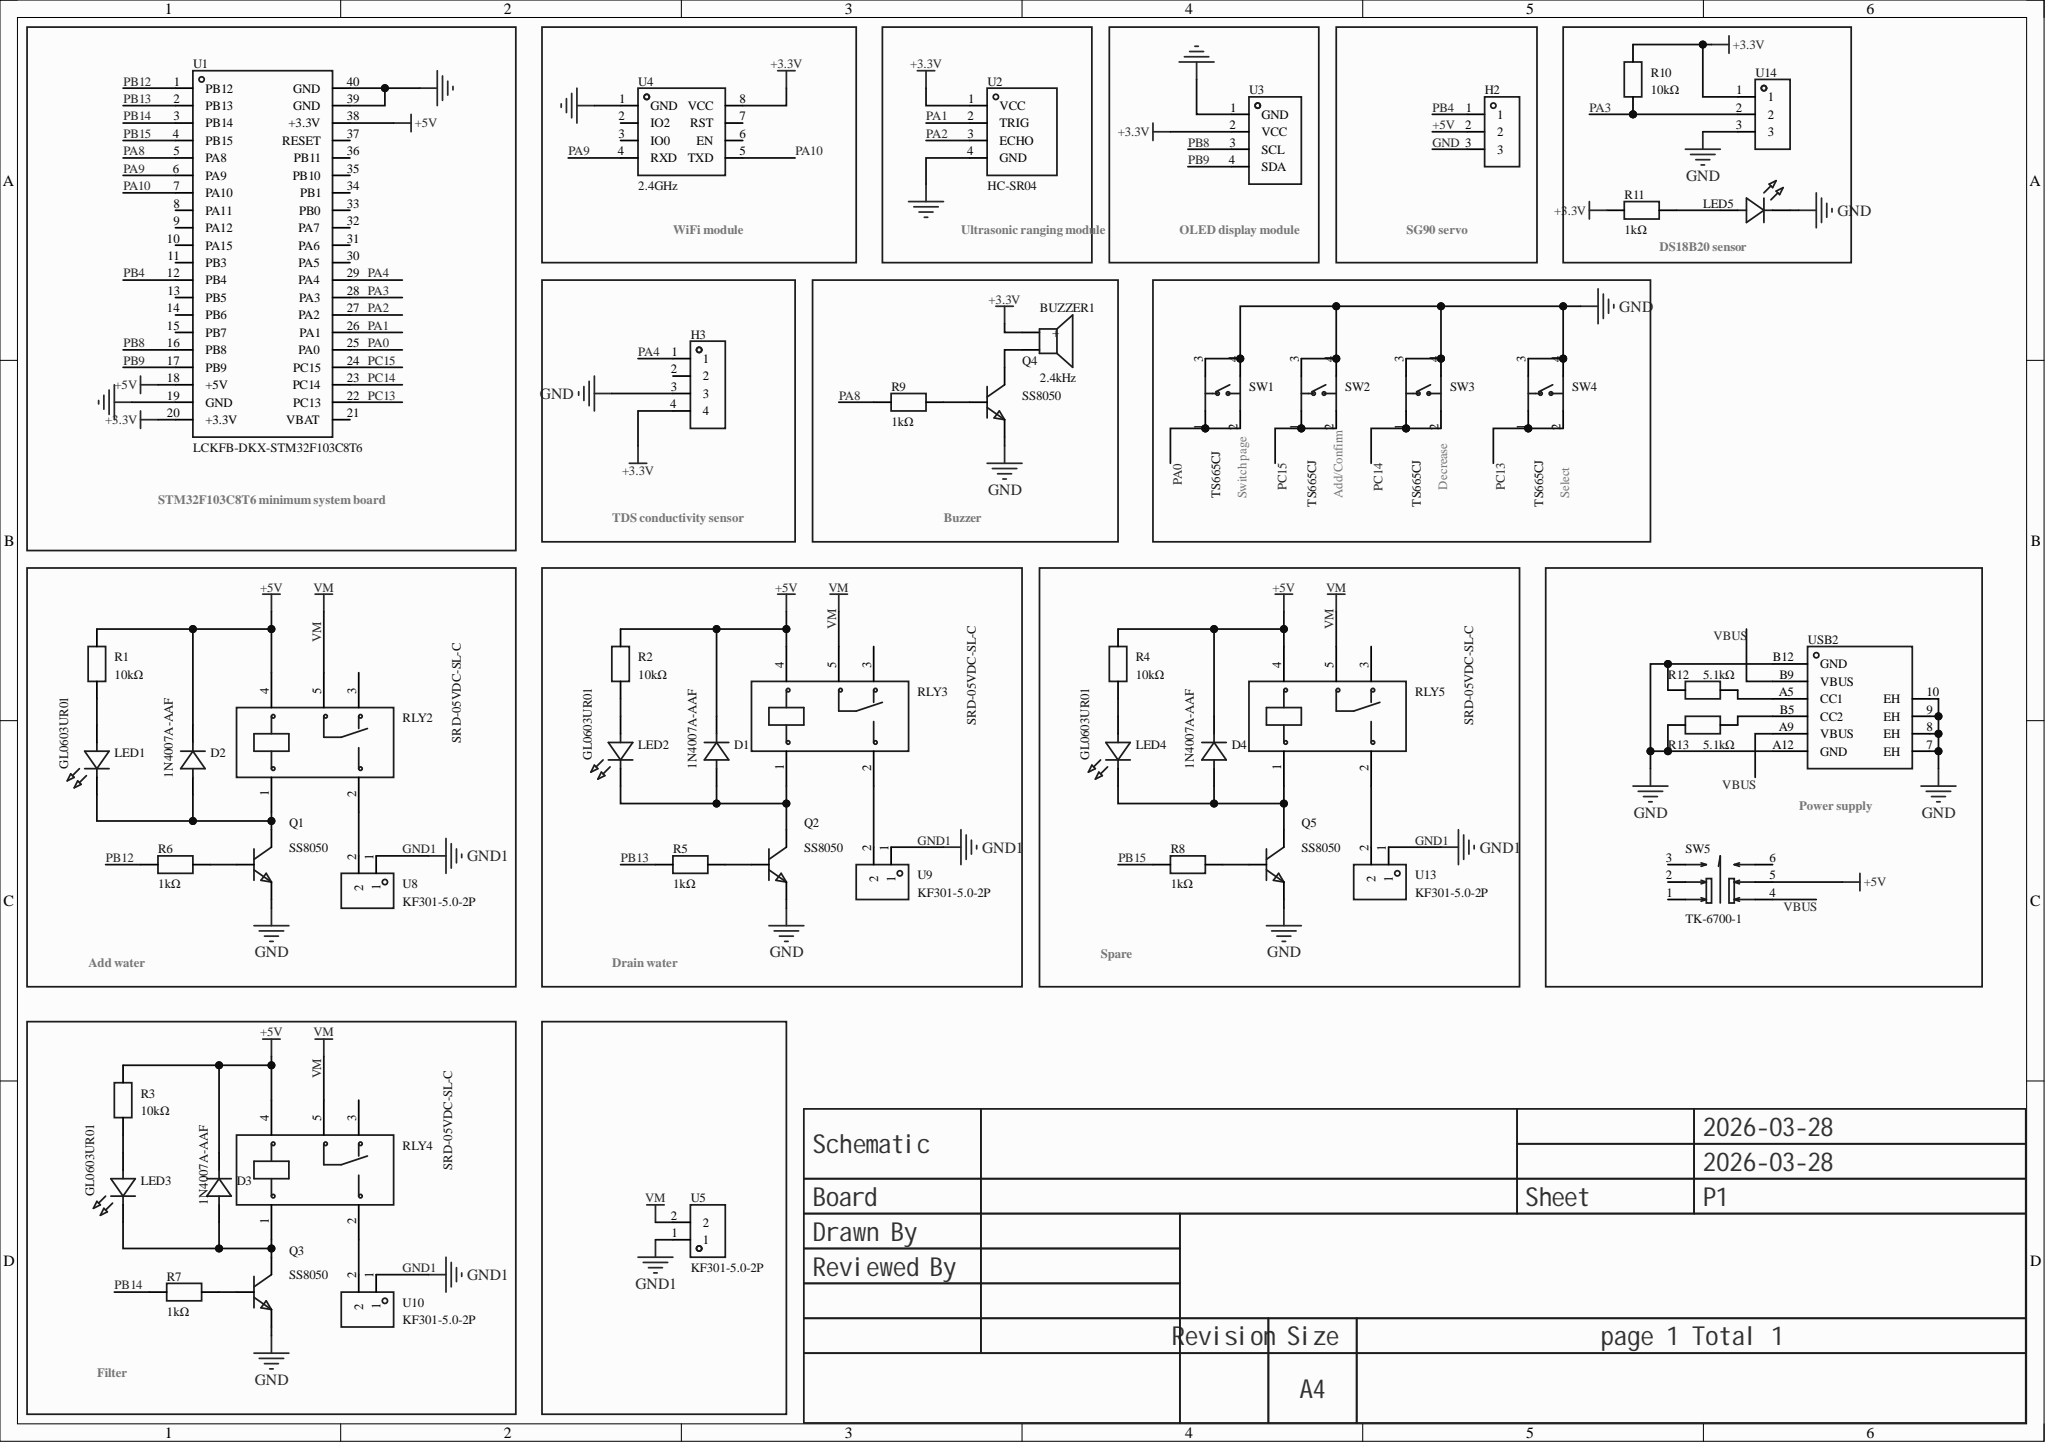Circuit board | Altium Designer | 50 parts | 45 nets
Bill of materials:
Comment,Description,Designator,Footprint,LibRef,Quantity
"2.4kHz","Drive mode: Active (built-in driver circuit); Construction: Electromagnetic; Rated voltage: 5V; Frequency: 2.4kHz; Sound pressure (SPL): 85dB;","BUZZER1","BUZ-TH_BD12.0-P7.60-D0.6-FD","TMB12A05_C96093","1"
"1N4007A-AAF","Diode configuration: Discrete; Forward voltage (Vf): 1.1V@1A; DC reverse voltage (Vr): 1kV; Rectifier current: 1A;","D1, D2, D3, D4","SMA_L4.3-W2.6-LS5.0-RD","1N4007A-AAF","4"
"PZ254V-11-03P","Pin structure: 1x3P; Pitch: 2.54mm; Row spacing: -; Round/square pin: Square pin; Mounting: Through-hole; Rows: Single row; Total pin count: 3P; Rated current: 3A; Rated voltage: 250V; Mating pin length: 6mm; Plastic height: 2.5mm; Termination pin length: 3mm; Operating temperature: -40℃~+105℃; Color: Black;","H2","HDR-TH_3P-P2.54-V-M_PZ254V-11-03P","PZ254V-11-03P","1"
"PZ254V-11-04P","Pin structure: 1x4P; Pitch: 2.54mm; Row spacing: -; Round/square pin: Square pin; Mounting: Through-hole; Rows: Single row; Total pin count: 4P; Rated current: 3A; Rated voltage: 250V; Mating pin length: 6mm; Plastic height: 2.5mm; Termination pin length: 3mm; Contact material: -; Operating temperature: -40℃~+105℃; Color: Black;","H3","HDR-TH_4P-P2.54-V-M","PZ254V-11-04P","1"
"GL0603UR01","Emitting color: Red; Forward voltage (Vf): 2.4V; Forward current: 20mA; Wavelength: 620nm~625nm; Diode configuration: Discrete diode; Lens color: Clear lens; Luminous intensity: 120mcd; Viewing angle: 120°; Packaging: Surface mount; Operating temperature: -40℃~+85℃;","LED1, LED2, LED3, LED4, LED5","LED0603-FD","GL0603UR01","5"
"SS8050","Transistor type: NPN; Collector current (Ic): 1.5A; Collector-emitter breakdown voltage (Vceo): 25V; Power dissipation (Pd): 300mW; DC current gain (hFE): 120@100mA,1.0V;","Q1, Q2, Q3, Q4, Q5","SOT-23-3_L2.9-W1.3-P1.90-LS2.4-BR","SS8050_C7420370","5"
"10kΩ","Resistor type: Metal film resistor; Resistance: 10kΩ; Tolerance: ±1%; Power: 250mW; Temperature coefficient: ±100ppm/?;","R1, R2, R3, R4, R10","RES-TH_BD2.7-L6.2-P10.20-D0.4","MF1/4W-10K±1%-ST52","5"
"1kΩ","Resistor type: Metal film resistor; Resistance: 1kΩ; Tolerance: ±1%; Power: 250mW; Temperature coefficient: ±100ppm/?;, Resistor type: Metal film resistor; Resistance: 10kΩ; Tolerance: ±1%; Power: 250mW; Temperature coefficient: ±100ppm/?;","R5, R6, R7, R8, R9, R11","RES-TH_BD2.7-L6.2-P10.20-D0.4","MF1/4W-1K±1%-ST52, MF1/4W-10K±1%-ST52","6"
"5.1kΩ","Resistor type: Metal film resistor; Resistance: 10kΩ; Tolerance: ±1%; Power: 250mW; Temperature coefficient: ±100ppm/?;","R12, R13","RES-TH_BD2.7-L6.2-P10.20-D0.4","MF1/4W-10K±1%-ST52","2"
"SRD-05VDC-SL-C","Coil voltage: 5V; Contact form: Changeover: 1C (SPDT); Contact rating (resistive load): -; Max switching voltage: 250V@AC; Max switching current: 15A;","RLY2, RLY3, RLY4, RLY5","RELAY-TH_SRD-XXVDC-XL-C","SRD-05VDC-SL-C","4"
"TS665CJ","Circuit structure: SPST; Button shape: Round button; Actuating force: 2.5N; Mounting: Through-hole; Switch length: 6mm; Switch width: 6mm; Switch height: 5mm; Bracket: Without bracket; Contact current: 50mA; Rated voltage: 12V; Lamp: None; Life: 5万 cycles;","SW1, SW2, SW3, SW4","SW-TH_4P-L6.0-W6.0-P4.50-LS6.5","TS665CJ","4"
"TK-6700-1","Circuit structure: DPDT; Self-locking/unlocking: Self-locking; Mounting: Through-hole; Actuating force: 2.3N; Operating life: -;","SW5","SW-TH_TK-6700-1","TK-6700-1","1"
"LCKFB-DKX-STM32F103C8T6","","U1","CONN-TH_L53.3-W22.9_STM32F103C8T6-CARD","LCKFB-DKX-STM32F103C8T6","1"
"HC-SR04","","U2","TH_HC-SR04V","HC-SR04","1"
"HS96L03W2C03","Controller chip: SSD1315; Interface type: I2C; Size (inch): 0.96; Pixel resolution: 128x64;","U3","OLED-TH_L27.8-W27.2-P2.54_C9900033791","HS96L03W2C03","1"
"2.4GHz","Core processor: ESP8266 chip; Frequency: 2.4GHz; Antenna type: On-board PCB antenna; TX power: 16dBm; RX sensitivity: -90dBm;","U4","WIFIM-TH_8P-L24.7-W14.4-P2.54","ESP-01S","1"
"KF301-5.0-2P","Structure: 1x2P; Pitch: 5mm; Color: Blue; Mounting: Through-hole; Rows: 1; Pins per row: 2; Rated current: 17A; Rated voltage: 250V; Wire gauge - AWG: 14~22; Wire gauge - mm²: 1.5; Operating temperature: -30℃~+120℃;","U5, U8, U9, U10, U13","CONN-TH_P5.00_KF301-5.0-2P","KF301-5.0-2P","5"
"WAFER-XH2.54-3PWZ","Pin structure: 1x3P; Pitch: 2.5mm; Mounting: Right angle; Reference series: XH; Total pin count: 3P; Rows: 1; Pins per row: 3; Row spacing: -; Rated current: 2A; Contact material: Brass; Contact plating: Tin; Operating temperature: -25℃~+85℃;","U14","CONN-TH_3P-P2.50_WAFER-XH2.54-3PWZ","WAFER-XH2.54-3PWZ","1"
"","","USB2","USB_ TYPE-C-6P","USB_ Type-C-6P","1"
Netlist (Protel format):
[
BUZZER1
BUZ-TH_BD12.0-P7.60-D0.6-FD
2.4kHz



]
[
D1
SMA_L4.3-W2.6-LS5.0-RD
1N4007A-AAF



]
[
D2
SMA_L4.3-W2.6-LS5.0-RD
1N4007A-AAF



]
[
D3
SMA_L4.3-W2.6-LS5.0-RD
1N4007A-AAF



]
[
D4
SMA_L4.3-W2.6-LS5.0-RD
1N4007A-AAF



]
[
H2
HDR-TH_3P-P2.54-V-M_PZ254V-11-03P
PZ254V-11-03P



]
[
H3
HDR-TH_4P-P2.54-V-M
PZ254V-11-04P



]
[
LED1
LED0603-FD
GL0603UR01



]
[
LED2
LED0603-FD
GL0603UR01



]
[
LED3
LED0603-FD
GL0603UR01



]
[
LED4
LED0603-FD
GL0603UR01



]
[
LED5
LED0603-FD
GL0603UR01



]
[
Q1
SOT-23-3_L2.9-W1.3-P1.90-LS2.4-BR
SS8050



]
[
Q2
SOT-23-3_L2.9-W1.3-P1.90-LS2.4-BR
SS8050



]
[
Q3
SOT-23-3_L2.9-W1.3-P1.90-LS2.4-BR
SS8050



]
[
Q4
SOT-23-3_L2.9-W1.3-P1.90-LS2.4-BR
SS8050



]
[
Q5
SOT-23-3_L2.9-W1.3-P1.90-LS2.4-BR
SS8050



]
[
R1
RES-TH_BD2.7-L6.2-P10.20-D0.4
10kΩ



]
[
R2
RES-TH_BD2.7-L6.2-P10.20-D0.4
10kΩ



]
[
R3
RES-TH_BD2.7-L6.2-P10.20-D0.4
10kΩ



]
[
R4
RES-TH_BD2.7-L6.2-P10.20-D0.4
10kΩ



]
[
R5
RES-TH_BD2.7-L6.2-P10.20-D0.4
1kΩ



]
[
R6
RES-TH_BD2.7-L6.2-P10.20-D0.4
1kΩ



]
[
R7
RES-TH_BD2.7-L6.2-P10.20-D0.4
1kΩ



]
[
R8
RES-TH_BD2.7-L6.2-P10.20-D0.4
1kΩ



]
[
R9
RES-TH_BD2.7-L6.2-P10.20-D0.4
1kΩ



]
[
R10
RES-TH_BD2.7-L6.2-P10.20-D0.4
10kΩ



]
[
R11
RES-TH_BD2.7-L6.2-P10.20-D0.4
1kΩ



]
[
R12
RES-TH_BD2.7-L6.2-P10.20-D0.4
5.1kΩ



]
[
R13
RES-TH_BD2.7-L6.2-P10.20-D0.4
5.1kΩ



]
[
RLY2
RELAY-TH_SRD-XXVDC-XL-C
SRD-05VDC-SL-C



]
[
RLY3
RELAY-TH_SRD-XXVDC-XL-C
SRD-05VDC-SL-C



]
[
RLY4
RELAY-TH_SRD-XXVDC-XL-C
SRD-05VDC-SL-C



]
[
RLY5
RELAY-TH_SRD-XXVDC-XL-C
SRD-05VDC-SL-C



]
[
SW1
SW-TH_4P-L6.0-W6.0-P4.50-LS6.5
TS665CJ



]
[
SW2
SW-TH_4P-L6.0-W6.0-P4.50-LS6.5
TS665CJ



]
[
SW3
SW-TH_4P-L6.0-W6.0-P4.50-LS6.5
TS665CJ



]
[
SW4
SW-TH_4P-L6.0-W6.0-P4.50-LS6.5
TS665CJ



]
[
SW5
SW-TH_TK-6700-1
TK-6700-1



]
[
U1
CONN-TH_L53.3-W22.9_STM32F103C8T6-CARD
LCKFB-DKX-STM32F103C8T6



]
[
U2
TH_HC-SR04V
HC-SR04



]
[
U3
OLED-TH_L27.8-W27.2-P2.54_C9900033791
HS96L03W2C03



]
[
U4
WIFIM-TH_8P-L24.7-W14.4-P2.54
2.4GHz



]
[
U5
CONN-TH_P5.00_KF301-5.0-2P
KF301-5.0-2P



]
[
U8
CONN-TH_P5.00_KF301-5.0-2P
KF301-5.0-2P



]
[
U9
CONN-TH_P5.00_KF301-5.0-2P
KF301-5.0-2P



]
[
U10
CONN-TH_P5.00_KF301-5.0-2P
KF301-5.0-2P



]
[
U13
CONN-TH_P5.00_KF301-5.0-2P
KF301-5.0-2P



]
[
U14
CONN-TH_3P-P2.50_WAFER-XH2.54-3PWZ
WAFER-XH2.54-3PWZ



]
[
USB2
USB_ TYPE-C-6P




]
(
VM
RLY2-5
RLY3-5
RLY4-5
RLY5-5
U5-2
)
(
VBUS
SW5-4
USB2-A9
USB2-B9
)
(
PC15
SW2-1
SW2-2
U1-24
)
(
PC14
SW3-1
SW3-2
U1-23
)
(
PC13
SW4-1
SW4-2
U1-22
)
(
PB15
R8-1
U1-4
)
(
PB14
R7-1
U1-3
)
(
PB13
R5-1
U1-2
)
(
PB12
R6-1
U1-1
)
(
PB9
U1-17
U3-4
)
(
PB8
U1-16
U3-3
)
(
PB4
H2-1
U1-12
)
(
PA10
U1-7
U4-5
)
(
PA9
U1-6
U4-4
)
(
PA8
R9-1
U1-5
)
(
PA4
H3-1
U1-29
)
(
PA3
R10-1
U1-28
U14-2
)
(
PA2
U1-27
U2-3
)
(
PA1
U1-26
U2-2
)
(
PA0
SW1-1
SW1-2
U1-25
)
(
NetRLY5_2
RLY5-2
U13-2
)
(
NetRLY4_2
RLY4-2
U10-2
)
(
NetRLY3_2
RLY3-2
U9-2
)
(
NetRLY2_2
RLY2-2
U8-2
)
(
NetR13_1
R13-1
USB2-B5
)
(
NetR12_2
R12-2
USB2-A5
)
(
NetQ5_1
Q5-1
R8-2
)
(
NetQ4_1
Q4-1
R9-2
)
(
NetQ3_1
Q3-1
R7-2
)
(
NetQ2_1
Q2-1
R5-2
)
(
NetQ1_1
Q1-1
R6-2
)
(
NetLED5_2
LED5-2
R11-1
)
(
NetLED4_2
LED4-2
R4-1
)
(
NetLED3_2
LED3-2
R3-1
)
(
NetLED2_2
LED2-2
R2-1
)
(
NetLED1_2
LED1-2
R1-1
)
(
NetD4_2
D4-2
LED4-1
Q5-3
RLY5-1
)
(
NetD3_2
D3-2
LED3-1
Q3-3
RLY4-1
)
(
NetD2_2
D2-2
LED1-1
Q1-3
RLY2-1
)
(
NetD1_2
D1-2
LED2-1
Q2-3
RLY3-1
)
(
NetBUZZER1_2
BUZZER1-2
Q4-3
)
(
GND1
U5-1
U8-1
U9-1
U10-1
U13-1
)
(
GND
H2-3
H3-3
LED5-1
Q1-2
Q2-2
Q3-2
Q4-2
Q5-2
R12-1
R13-2
SW1-3
SW1-4
SW2-3
SW2-4
SW3-3
SW3-4
SW4-3
SW4-4
U1-19
U1-39
U1-40
U2-4
U3-1
U4-1
U14-3
USB2-7
USB2-8
USB2-9
USB2-10
USB2-A12
USB2-B12
)
(
+5V
D1-1
D2-1
D3-1
D4-1
H2-2
R1-2
R2-2
R3-2
R4-2
RLY2-4
RLY3-4
RLY4-4
RLY5-4
SW5-5
U1-18
U1-38
)
(
+3.3V
BUZZER1-1
H3-4
R10-2
R11-2
U1-20
U2-1
U3-2
U4-8
U14-1
)